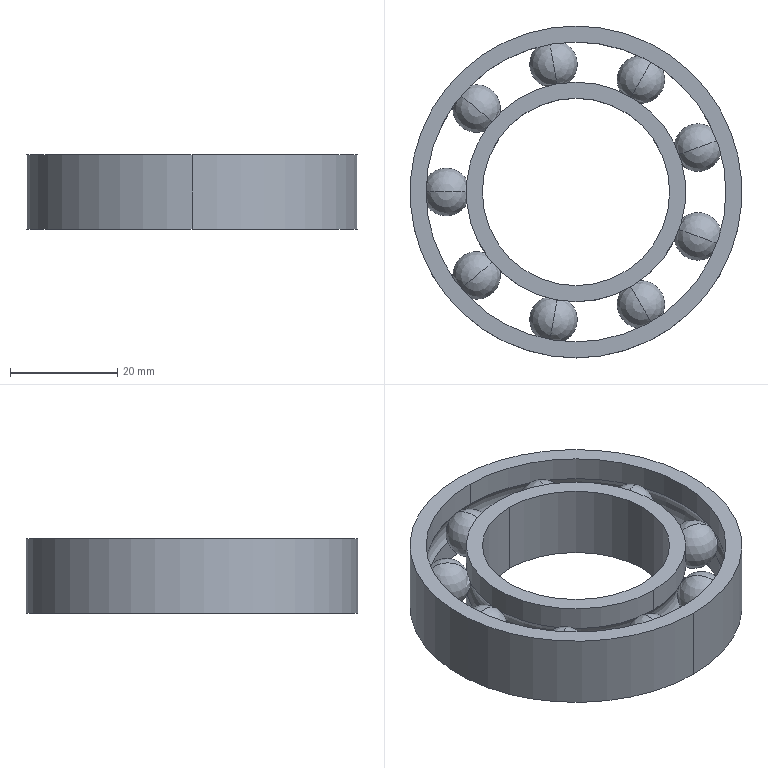Part | NX | features BREP 11 | 11 solids | 38 faces | box 62 x 62 x 14 mm | volume 15463 mm3 | sphere 18 | cylinder 12 | plane 4 | torus 4 | commonest cylinder face diameters 41 x4 56 x4 35 x2 62 x2
STEP:
#1=CARTESIAN_POINT('',(-18.577,15.588,-4.5));
#2=VERTEX_POINT('',#1);
#3=CARTESIAN_POINT('',(-18.577,15.588,4.5));
#4=VERTEX_POINT('',#3);
#5=CARTESIAN_POINT('',(-18.577,15.588,0.));
#6=DIRECTION('',(-0.6428,-0.766,0.));
#7=DIRECTION('',(0.,0.,-1.));
#8=AXIS2_PLACEMENT_3D('',#5,#6,#7);
#9=CIRCLE('',#8,4.5);
#10=EDGE_CURVE('',#2,#4,#9,.T.);
#11=ORIENTED_EDGE('',*,*,#10,.F.);
#12=CARTESIAN_POINT('',(-18.577,15.588,0.));
#13=DIRECTION('',(0.6428,0.766,0.));
#14=DIRECTION('',(0.,0.,-1.));
#15=AXIS2_PLACEMENT_3D('',#12,#13,#14);
#16=CIRCLE('',#15,4.5);
#17=EDGE_CURVE('',#2,#4,#16,.T.);
#18=ORIENTED_EDGE('',*,*,#17,.T.);
#19=EDGE_LOOP('',(#11,#18));
#20=FACE_BOUND('',#19,.T.);
#21=CARTESIAN_POINT('',(-18.577,15.588,0.));
#22=DIRECTION('',(0.,0.,-1.));
#23=DIRECTION('',(-0.766,0.6428,0.));
#24=AXIS2_PLACEMENT_3D('',#21,#22,#23);
#25=SPHERICAL_SURFACE('',#24,4.5);
#26=ADVANCED_FACE('',(#20),#25,.T.);
#27=ORIENTED_EDGE('',*,*,#10,.T.);
#28=ORIENTED_EDGE('',*,*,#17,.F.);
#29=EDGE_LOOP('',(#27,#28));
#30=FACE_BOUND('',#29,.T.);
#31=CARTESIAN_POINT('',(-18.577,15.588,0.));
#32=DIRECTION('',(0.,0.,-1.));
#33=DIRECTION('',(-0.766,0.6428,0.));
#34=AXIS2_PLACEMENT_3D('',#31,#32,#33);
#35=SPHERICAL_SURFACE('',#34,4.5);
#36=ADVANCED_FACE('',(#30),#35,.T.);
#37=CLOSED_SHELL('',(#26,#36));
#38=MANIFOLD_SOLID_BREP('',#37);
#39=CARTESIAN_POINT('',(-4.211,23.882,-4.5));
#40=VERTEX_POINT('',#39);
#41=CARTESIAN_POINT('',(-4.211,23.882,4.5));
#42=VERTEX_POINT('',#41);
#43=CARTESIAN_POINT('',(-4.211,23.882,0.));
#44=DIRECTION('',(-0.9848,-0.1736,0.));
#45=DIRECTION('',(0.,0.,-1.));
#46=AXIS2_PLACEMENT_3D('',#43,#44,#45);
#47=CIRCLE('',#46,4.5);
#48=EDGE_CURVE('',#40,#42,#47,.T.);
#49=ORIENTED_EDGE('',*,*,#48,.F.);
#50=CARTESIAN_POINT('',(-4.211,23.882,0.));
#51=DIRECTION('',(0.9848,0.1736,0.));
#52=DIRECTION('',(0.,0.,-1.));
#53=AXIS2_PLACEMENT_3D('',#50,#51,#52);
#54=CIRCLE('',#53,4.5);
#55=EDGE_CURVE('',#40,#42,#54,.T.);
#56=ORIENTED_EDGE('',*,*,#55,.T.);
#57=EDGE_LOOP('',(#49,#56));
#58=FACE_BOUND('',#57,.T.);
#59=CARTESIAN_POINT('',(-4.211,23.882,0.));
#60=DIRECTION('',(0.,0.,-1.));
#61=DIRECTION('',(-0.1736,0.9848,0.));
#62=AXIS2_PLACEMENT_3D('',#59,#60,#61);
#63=SPHERICAL_SURFACE('',#62,4.5);
#64=ADVANCED_FACE('',(#58),#63,.T.);
#65=ORIENTED_EDGE('',*,*,#48,.T.);
#66=ORIENTED_EDGE('',*,*,#55,.F.);
#67=EDGE_LOOP('',(#65,#66));
#68=FACE_BOUND('',#67,.T.);
#69=CARTESIAN_POINT('',(-4.211,23.882,0.));
#70=DIRECTION('',(0.,0.,-1.));
#71=DIRECTION('',(-0.1736,0.9848,0.));
#72=AXIS2_PLACEMENT_3D('',#69,#70,#71);
#73=SPHERICAL_SURFACE('',#72,4.5);
#74=ADVANCED_FACE('',(#68),#73,.T.);
#75=CLOSED_SHELL('',(#64,#74));
#76=MANIFOLD_SOLID_BREP('',#75);
#77=CARTESIAN_POINT('',(0.,31.,-7.));
#78=VERTEX_POINT('',#77);
#79=CARTESIAN_POINT('',(0.,-31.,-7.));
#80=VERTEX_POINT('',#79);
#81=CARTESIAN_POINT('',(0.,0.,-7.));
#82=DIRECTION('',(0.,0.,1.));
#83=DIRECTION('',(0.,1.,0.));
#84=AXIS2_PLACEMENT_3D('',#81,#82,#83);
#85=CIRCLE('',#84,31.);
#86=EDGE_CURVE('',#78,#80,#85,.T.);
#87=ORIENTED_EDGE('',*,*,#86,.T.);
#88=CARTESIAN_POINT('',(0.,-31.,7.));
#89=VERTEX_POINT('',#88);
#90=CARTESIAN_POINT('',(0.,-31.,-7.));
#91=DIRECTION('',(0.,0.,1.));
#92=VECTOR('',#91,1000.);
#93=LINE('',#90,#92);
#94=EDGE_CURVE('',#80,#89,#93,.T.);
#95=ORIENTED_EDGE('',*,*,#94,.T.);
#96=CARTESIAN_POINT('',(0.,31.,7.));
#97=VERTEX_POINT('',#96);
#98=CARTESIAN_POINT('',(0.,0.,7.));
#99=DIRECTION('',(0.,0.,1.));
#100=DIRECTION('',(0.,1.,0.));
#101=AXIS2_PLACEMENT_3D('',#98,#99,#100);
#102=CIRCLE('',#101,31.);
#103=EDGE_CURVE('',#97,#89,#102,.T.);
#104=ORIENTED_EDGE('',*,*,#103,.F.);
#105=CARTESIAN_POINT('',(0.,31.,-7.));
#106=DIRECTION('',(0.,0.,1.));
#107=VECTOR('',#106,1000.);
#108=LINE('',#105,#107);
#109=EDGE_CURVE('',#78,#97,#108,.T.);
#110=ORIENTED_EDGE('',*,*,#109,.F.);
#111=EDGE_LOOP('',(#87,#95,#104,#110));
#112=FACE_BOUND('',#111,.T.);
#113=CARTESIAN_POINT('',(0.,0.,7.7));
#114=DIRECTION('',(0.,0.,-1.));
#115=DIRECTION('',(0.,1.,0.));
#116=AXIS2_PLACEMENT_3D('',#113,#114,#115);
#117=CYLINDRICAL_SURFACE('',#116,31.);
#118=ADVANCED_FACE('',(#112),#117,.T.);
#119=CARTESIAN_POINT('',(0.,0.,7.));
#120=DIRECTION('',(0.,0.,-1.));
#121=DIRECTION('',(0.,1.,0.));
#122=AXIS2_PLACEMENT_3D('',#119,#120,#121);
#123=CIRCLE('',#122,31.);
#124=EDGE_CURVE('',#97,#89,#123,.T.);
#125=ORIENTED_EDGE('',*,*,#124,.T.);
#126=ORIENTED_EDGE('',*,*,#94,.F.);
#127=CARTESIAN_POINT('',(0.,0.,-7.));
#128=DIRECTION('',(0.,0.,-1.));
#129=DIRECTION('',(0.,1.,0.));
#130=AXIS2_PLACEMENT_3D('',#127,#128,#129);
#131=CIRCLE('',#130,31.);
#132=EDGE_CURVE('',#78,#80,#131,.T.);
#133=ORIENTED_EDGE('',*,*,#132,.F.);
#134=ORIENTED_EDGE('',*,*,#109,.T.);
#135=EDGE_LOOP('',(#125,#126,#133,#134));
#136=FACE_BOUND('',#135,.T.);
#137=CARTESIAN_POINT('',(0.,0.,7.7));
#138=DIRECTION('',(0.,0.,-1.));
#139=DIRECTION('',(0.,1.,0.));
#140=AXIS2_PLACEMENT_3D('',#137,#138,#139);
#141=CYLINDRICAL_SURFACE('',#140,31.);
#142=ADVANCED_FACE('',(#136),#141,.T.);
#143=ORIENTED_EDGE('',*,*,#86,.F.);
#144=ORIENTED_EDGE('',*,*,#132,.T.);
#145=EDGE_LOOP('',(#143,#144));
#146=FACE_BOUND('',#145,.T.);
#147=CARTESIAN_POINT('',(0.,28.,-7.));
#148=VERTEX_POINT('',#147);
#149=CARTESIAN_POINT('',(0.,-28.,-7.));
#150=VERTEX_POINT('',#149);
#151=CARTESIAN_POINT('',(0.,0.,-7.));
#152=DIRECTION('',(0.,0.,-1.));
#153=DIRECTION('',(0.,1.,0.));
#154=AXIS2_PLACEMENT_3D('',#151,#152,#153);
#155=CIRCLE('',#154,28.);
#156=EDGE_CURVE('',#148,#150,#155,.T.);
#157=ORIENTED_EDGE('',*,*,#156,.F.);
#158=CARTESIAN_POINT('',(0.,0.,-7.));
#159=DIRECTION('',(0.,0.,1.));
#160=DIRECTION('',(0.,1.,0.));
#161=AXIS2_PLACEMENT_3D('',#158,#159,#160);
#162=CIRCLE('',#161,28.);
#163=EDGE_CURVE('',#148,#150,#162,.T.);
#164=ORIENTED_EDGE('',*,*,#163,.T.);
#165=EDGE_LOOP('',(#157,#164));
#166=FACE_BOUND('',#165,.T.);
#167=CARTESIAN_POINT('',(0.,0.,-7.));
#168=DIRECTION('',(0.,0.,-1.));
#169=DIRECTION('',(0.,1.,0.));
#170=AXIS2_PLACEMENT_3D('',#167,#168,#169);
#171=PLANE('',#170);
#172=ADVANCED_FACE('',(#146,#166),#171,.T.);
#173=CARTESIAN_POINT('',(0.,28.,-2.487));
#174=VERTEX_POINT('',#173);
#175=CARTESIAN_POINT('',(0.,-28.,-2.487));
#176=VERTEX_POINT('',#175);
#177=CARTESIAN_POINT('',(0.,0.,-2.487));
#178=DIRECTION('',(0.,0.,1.));
#179=DIRECTION('',(0.,1.,0.));
#180=AXIS2_PLACEMENT_3D('',#177,#178,#179);
#181=CIRCLE('',#180,28.);
#182=EDGE_CURVE('',#174,#176,#181,.T.);
#183=ORIENTED_EDGE('',*,*,#182,.T.);
#184=CARTESIAN_POINT('',(0.,-28.,-2.487));
#185=DIRECTION('',(0.,0.,-1.));
#186=VECTOR('',#185,1000.);
#187=LINE('',#184,#186);
#188=EDGE_CURVE('',#176,#150,#187,.T.);
#189=ORIENTED_EDGE('',*,*,#188,.T.);
#190=ORIENTED_EDGE('',*,*,#163,.F.);
#191=CARTESIAN_POINT('',(0.,28.,-2.487));
#192=DIRECTION('',(0.,0.,-1.));
#193=VECTOR('',#192,1000.);
#194=LINE('',#191,#193);
#195=EDGE_CURVE('',#174,#148,#194,.T.);
#196=ORIENTED_EDGE('',*,*,#195,.F.);
#197=EDGE_LOOP('',(#183,#189,#190,#196));
#198=FACE_BOUND('',#197,.T.);
#199=CARTESIAN_POINT('',(0.,0.,7.7));
#200=DIRECTION('',(0.,0.,-1.));
#201=DIRECTION('',(0.,1.,0.));
#202=AXIS2_PLACEMENT_3D('',#199,#200,#201);
#203=CYLINDRICAL_SURFACE('',#202,28.);
#204=ADVANCED_FACE('',(#198),#203,.F.);
#205=ORIENTED_EDGE('',*,*,#156,.T.);
#206=ORIENTED_EDGE('',*,*,#188,.F.);
#207=CARTESIAN_POINT('',(0.,0.,-2.487));
#208=DIRECTION('',(0.,0.,-1.));
#209=DIRECTION('',(0.,1.,0.));
#210=AXIS2_PLACEMENT_3D('',#207,#208,#209);
#211=CIRCLE('',#210,28.);
#212=EDGE_CURVE('',#174,#176,#211,.T.);
#213=ORIENTED_EDGE('',*,*,#212,.F.);
#214=ORIENTED_EDGE('',*,*,#195,.T.);
#215=EDGE_LOOP('',(#205,#206,#213,#214));
#216=FACE_BOUND('',#215,.T.);
#217=CARTESIAN_POINT('',(0.,0.,7.7));
#218=DIRECTION('',(0.,0.,-1.));
#219=DIRECTION('',(0.,1.,0.));
#220=AXIS2_PLACEMENT_3D('',#217,#218,#219);
#221=CYLINDRICAL_SURFACE('',#220,28.);
#222=ADVANCED_FACE('',(#216),#221,.F.);
#223=ORIENTED_EDGE('',*,*,#212,.T.);
#224=CARTESIAN_POINT('',(0.,-28.,2.487));
#225=VERTEX_POINT('',#224);
#226=CARTESIAN_POINT('',(0.,-24.25,0.));
#227=DIRECTION('',(1.,0.,0.));
#228=DIRECTION('',(0.,-0.8333,0.5528));
#229=AXIS2_PLACEMENT_3D('',#226,#227,#228);
#230=CIRCLE('',#229,4.5);
#231=EDGE_CURVE('',#176,#225,#230,.F.);
#232=ORIENTED_EDGE('',*,*,#231,.T.);
#233=CARTESIAN_POINT('',(0.,28.,2.487));
#234=VERTEX_POINT('',#233);
#235=CARTESIAN_POINT('',(0.,0.,2.487));
#236=DIRECTION('',(0.,0.,-1.));
#237=DIRECTION('',(0.,1.,0.));
#238=AXIS2_PLACEMENT_3D('',#235,#236,#237);
#239=CIRCLE('',#238,28.);
#240=EDGE_CURVE('',#234,#225,#239,.T.);
#241=ORIENTED_EDGE('',*,*,#240,.F.);
#242=CARTESIAN_POINT('',(0.,24.25,0.));
#243=DIRECTION('',(-1.,0.,0.));
#244=DIRECTION('',(0.,0.8333,0.5528));
#245=AXIS2_PLACEMENT_3D('',#242,#243,#244);
#246=CIRCLE('',#245,4.5);
#247=EDGE_CURVE('',#174,#234,#246,.F.);
#248=ORIENTED_EDGE('',*,*,#247,.F.);
#249=EDGE_LOOP('',(#223,#232,#241,#248));
#250=FACE_BOUND('',#249,.T.);
#251=CARTESIAN_POINT('',(0.,0.,0.));
#252=DIRECTION('',(0.,0.,-1.));
#253=DIRECTION('',(0.,1.,0.));
#254=AXIS2_PLACEMENT_3D('',#251,#252,#253);
#255=TOROIDAL_SURFACE('',#254,24.25,4.5);
#256=ADVANCED_FACE('',(#250),#255,.F.);
#257=CARTESIAN_POINT('',(0.,0.,2.487));
#258=DIRECTION('',(0.,0.,1.));
#259=DIRECTION('',(0.,1.,0.));
#260=AXIS2_PLACEMENT_3D('',#257,#258,#259);
#261=CIRCLE('',#260,28.);
#262=EDGE_CURVE('',#234,#225,#261,.T.);
#263=ORIENTED_EDGE('',*,*,#262,.T.);
#264=ORIENTED_EDGE('',*,*,#231,.F.);
#265=ORIENTED_EDGE('',*,*,#182,.F.);
#266=ORIENTED_EDGE('',*,*,#247,.T.);
#267=EDGE_LOOP('',(#263,#264,#265,#266));
#268=FACE_BOUND('',#267,.T.);
#269=CARTESIAN_POINT('',(0.,0.,0.));
#270=DIRECTION('',(0.,0.,-1.));
#271=DIRECTION('',(0.,1.,0.));
#272=AXIS2_PLACEMENT_3D('',#269,#270,#271);
#273=TOROIDAL_SURFACE('',#272,24.25,4.5);
#274=ADVANCED_FACE('',(#268),#273,.F.);
#275=CARTESIAN_POINT('',(0.,28.,7.));
#276=VERTEX_POINT('',#275);
#277=CARTESIAN_POINT('',(0.,-28.,7.));
#278=VERTEX_POINT('',#277);
#279=CARTESIAN_POINT('',(0.,0.,7.));
#280=DIRECTION('',(0.,0.,1.));
#281=DIRECTION('',(0.,1.,0.));
#282=AXIS2_PLACEMENT_3D('',#279,#280,#281);
#283=CIRCLE('',#282,28.);
#284=EDGE_CURVE('',#276,#278,#283,.T.);
#285=ORIENTED_EDGE('',*,*,#284,.T.);
#286=CARTESIAN_POINT('',(0.,-28.,7.));
#287=DIRECTION('',(0.,0.,-1.));
#288=VECTOR('',#287,1000.);
#289=LINE('',#286,#288);
#290=EDGE_CURVE('',#278,#225,#289,.T.);
#291=ORIENTED_EDGE('',*,*,#290,.T.);
#292=ORIENTED_EDGE('',*,*,#262,.F.);
#293=CARTESIAN_POINT('',(0.,28.,7.));
#294=DIRECTION('',(0.,0.,-1.));
#295=VECTOR('',#294,1000.);
#296=LINE('',#293,#295);
#297=EDGE_CURVE('',#276,#234,#296,.T.);
#298=ORIENTED_EDGE('',*,*,#297,.F.);
#299=EDGE_LOOP('',(#285,#291,#292,#298));
#300=FACE_BOUND('',#299,.T.);
#301=CARTESIAN_POINT('',(0.,0.,7.7));
#302=DIRECTION('',(0.,0.,-1.));
#303=DIRECTION('',(0.,1.,0.));
#304=AXIS2_PLACEMENT_3D('',#301,#302,#303);
#305=CYLINDRICAL_SURFACE('',#304,28.);
#306=ADVANCED_FACE('',(#300),#305,.F.);
#307=ORIENTED_EDGE('',*,*,#240,.T.);
#308=ORIENTED_EDGE('',*,*,#290,.F.);
#309=CARTESIAN_POINT('',(0.,0.,7.));
#310=DIRECTION('',(0.,0.,-1.));
#311=DIRECTION('',(0.,1.,0.));
#312=AXIS2_PLACEMENT_3D('',#309,#310,#311);
#313=CIRCLE('',#312,28.);
#314=EDGE_CURVE('',#276,#278,#313,.T.);
#315=ORIENTED_EDGE('',*,*,#314,.F.);
#316=ORIENTED_EDGE('',*,*,#297,.T.);
#317=EDGE_LOOP('',(#307,#308,#315,#316));
#318=FACE_BOUND('',#317,.T.);
#319=CARTESIAN_POINT('',(0.,0.,7.7));
#320=DIRECTION('',(0.,0.,-1.));
#321=DIRECTION('',(0.,1.,0.));
#322=AXIS2_PLACEMENT_3D('',#319,#320,#321);
#323=CYLINDRICAL_SURFACE('',#322,28.);
#324=ADVANCED_FACE('',(#318),#323,.F.);
#325=ORIENTED_EDGE('',*,*,#124,.F.);
#326=ORIENTED_EDGE('',*,*,#103,.T.);
#327=EDGE_LOOP('',(#325,#326));
#328=FACE_BOUND('',#327,.T.);
#329=ORIENTED_EDGE('',*,*,#284,.F.);
#330=ORIENTED_EDGE('',*,*,#314,.T.);
#331=EDGE_LOOP('',(#329,#330));
#332=FACE_BOUND('',#331,.T.);
#333=CARTESIAN_POINT('',(0.,0.,7.));
#334=DIRECTION('',(0.,0.,-1.));
#335=DIRECTION('',(0.,1.,0.));
#336=AXIS2_PLACEMENT_3D('',#333,#334,#335);
#337=PLANE('',#336);
#338=ADVANCED_FACE('',(#328,#332),#337,.F.);
#339=CLOSED_SHELL('',(#118,#142,#172,#204,#222,#256,#274,#306,#324,#338));
#340=MANIFOLD_SOLID_BREP('',#339);
#341=CARTESIAN_POINT('',(12.125,21.001,4.5));
#342=VERTEX_POINT('',#341);
#343=CARTESIAN_POINT('',(12.125,21.001,-4.5));
#344=VERTEX_POINT('',#343);
#345=CARTESIAN_POINT('',(12.125,21.001,0.));
#346=DIRECTION('',(-0.866,0.5,0.));
#347=DIRECTION('',(0.,0.,-1.));
#348=AXIS2_PLACEMENT_3D('',#345,#346,#347);
#349=CIRCLE('',#348,4.5);
#350=EDGE_CURVE('',#342,#344,#349,.F.);
#351=ORIENTED_EDGE('',*,*,#350,.T.);
#352=CARTESIAN_POINT('',(12.125,21.001,0.));
#353=DIRECTION('',(0.866,-0.5,0.));
#354=DIRECTION('',(0.,0.,-1.));
#355=AXIS2_PLACEMENT_3D('',#352,#353,#354);
#356=CIRCLE('',#355,4.5);
#357=EDGE_CURVE('',#342,#344,#356,.F.);
#358=ORIENTED_EDGE('',*,*,#357,.F.);
#359=EDGE_LOOP('',(#351,#358));
#360=FACE_BOUND('',#359,.T.);
#361=CARTESIAN_POINT('',(12.125,21.001,0.));
#362=DIRECTION('',(0.,0.,-1.));
#363=DIRECTION('',(0.5,0.866,0.));
#364=AXIS2_PLACEMENT_3D('',#361,#362,#363);
#365=SPHERICAL_SURFACE('',#364,4.5);
#366=ADVANCED_FACE('',(#360),#365,.T.);
#367=ORIENTED_EDGE('',*,*,#350,.F.);
#368=ORIENTED_EDGE('',*,*,#357,.T.);
#369=EDGE_LOOP('',(#367,#368));
#370=FACE_BOUND('',#369,.T.);
#371=CARTESIAN_POINT('',(12.125,21.001,0.));
#372=DIRECTION('',(0.,0.,-1.));
#373=DIRECTION('',(0.5,0.866,0.));
#374=AXIS2_PLACEMENT_3D('',#371,#372,#373);
#375=SPHERICAL_SURFACE('',#374,4.5);
#376=ADVANCED_FACE('',(#370),#375,.T.);
#377=CLOSED_SHELL('',(#366,#376));
#378=MANIFOLD_SOLID_BREP('',#377);
#379=CARTESIAN_POINT('',(0.,20.5,2.487));
#380=VERTEX_POINT('',#379);
#381=CARTESIAN_POINT('',(0.,-20.5,2.487));
#382=VERTEX_POINT('',#381);
#383=CARTESIAN_POINT('',(0.,0.,2.487));
#384=DIRECTION('',(0.,0.,1.));
#385=DIRECTION('',(0.,1.,0.));
#386=AXIS2_PLACEMENT_3D('',#383,#384,#385);
#387=CIRCLE('',#386,20.5);
#388=EDGE_CURVE('',#380,#382,#387,.T.);
#389=ORIENTED_EDGE('',*,*,#388,.T.);
#390=CARTESIAN_POINT('',(0.,-20.5,7.));
#391=VERTEX_POINT('',#390);
#392=CARTESIAN_POINT('',(0.,-20.5,2.487));
#393=DIRECTION('',(0.,0.,1.));
#394=VECTOR('',#393,1000.);
#395=LINE('',#392,#394);
#396=EDGE_CURVE('',#382,#391,#395,.T.);
#397=ORIENTED_EDGE('',*,*,#396,.T.);
#398=CARTESIAN_POINT('',(0.,20.5,7.));
#399=VERTEX_POINT('',#398);
#400=CARTESIAN_POINT('',(0.,0.,7.));
#401=DIRECTION('',(0.,0.,1.));
#402=DIRECTION('',(0.,1.,0.));
#403=AXIS2_PLACEMENT_3D('',#400,#401,#402);
#404=CIRCLE('',#403,20.5);
#405=EDGE_CURVE('',#399,#391,#404,.T.);
#406=ORIENTED_EDGE('',*,*,#405,.F.);
#407=CARTESIAN_POINT('',(0.,20.5,2.487));
#408=DIRECTION('',(0.,0.,1.));
#409=VECTOR('',#408,1000.);
#410=LINE('',#407,#409);
#411=EDGE_CURVE('',#380,#399,#410,.T.);
#412=ORIENTED_EDGE('',*,*,#411,.F.);
#413=EDGE_LOOP('',(#389,#397,#406,#412));
#414=FACE_BOUND('',#413,.T.);
#415=CARTESIAN_POINT('',(0.,0.,7.7));
#416=DIRECTION('',(0.,0.,-1.));
#417=DIRECTION('',(0.,1.,0.));
#418=AXIS2_PLACEMENT_3D('',#415,#416,#417);
#419=CYLINDRICAL_SURFACE('',#418,20.5);
#420=ADVANCED_FACE('',(#414),#419,.T.);
#421=CARTESIAN_POINT('',(0.,0.,7.));
#422=DIRECTION('',(0.,0.,-1.));
#423=DIRECTION('',(0.,1.,0.));
#424=AXIS2_PLACEMENT_3D('',#421,#422,#423);
#425=CIRCLE('',#424,20.5);
#426=EDGE_CURVE('',#399,#391,#425,.T.);
#427=ORIENTED_EDGE('',*,*,#426,.T.);
#428=ORIENTED_EDGE('',*,*,#396,.F.);
#429=CARTESIAN_POINT('',(0.,0.,2.487));
#430=DIRECTION('',(0.,0.,-1.));
#431=DIRECTION('',(0.,1.,0.));
#432=AXIS2_PLACEMENT_3D('',#429,#430,#431);
#433=CIRCLE('',#432,20.5);
#434=EDGE_CURVE('',#380,#382,#433,.T.);
#435=ORIENTED_EDGE('',*,*,#434,.F.);
#436=ORIENTED_EDGE('',*,*,#411,.T.);
#437=EDGE_LOOP('',(#427,#428,#435,#436));
#438=FACE_BOUND('',#437,.T.);
#439=CARTESIAN_POINT('',(0.,0.,7.7));
#440=DIRECTION('',(0.,0.,-1.));
#441=DIRECTION('',(0.,1.,0.));
#442=AXIS2_PLACEMENT_3D('',#439,#440,#441);
#443=CYLINDRICAL_SURFACE('',#442,20.5);
#444=ADVANCED_FACE('',(#438),#443,.T.);
#445=ORIENTED_EDGE('',*,*,#434,.T.);
#446=CARTESIAN_POINT('',(0.,-20.5,-2.487));
#447=VERTEX_POINT('',#446);
#448=CARTESIAN_POINT('',(0.,-24.25,0.));
#449=DIRECTION('',(1.,0.,0.));
#450=DIRECTION('',(0.,0.8333,-0.5528));
#451=AXIS2_PLACEMENT_3D('',#448,#449,#450);
#452=CIRCLE('',#451,4.5);
#453=EDGE_CURVE('',#382,#447,#452,.F.);
#454=ORIENTED_EDGE('',*,*,#453,.T.);
#455=CARTESIAN_POINT('',(0.,20.5,-2.487));
#456=VERTEX_POINT('',#455);
#457=CARTESIAN_POINT('',(0.,0.,-2.487));
#458=DIRECTION('',(0.,0.,-1.));
#459=DIRECTION('',(0.,1.,0.));
#460=AXIS2_PLACEMENT_3D('',#457,#458,#459);
#461=CIRCLE('',#460,20.5);
#462=EDGE_CURVE('',#456,#447,#461,.T.);
#463=ORIENTED_EDGE('',*,*,#462,.F.);
#464=CARTESIAN_POINT('',(0.,24.25,0.));
#465=DIRECTION('',(-1.,0.,0.));
#466=DIRECTION('',(0.,-0.8333,-0.5528));
#467=AXIS2_PLACEMENT_3D('',#464,#465,#466);
#468=CIRCLE('',#467,4.5);
#469=EDGE_CURVE('',#380,#456,#468,.F.);
#470=ORIENTED_EDGE('',*,*,#469,.F.);
#471=EDGE_LOOP('',(#445,#454,#463,#470));
#472=FACE_BOUND('',#471,.T.);
#473=CARTESIAN_POINT('',(0.,0.,0.));
#474=DIRECTION('',(0.,0.,-1.));
#475=DIRECTION('',(0.,1.,0.));
#476=AXIS2_PLACEMENT_3D('',#473,#474,#475);
#477=TOROIDAL_SURFACE('',#476,24.25,4.5);
#478=ADVANCED_FACE('',(#472),#477,.F.);
#479=CARTESIAN_POINT('',(0.,0.,-2.487));
#480=DIRECTION('',(0.,0.,1.));
#481=DIRECTION('',(0.,1.,0.));
#482=AXIS2_PLACEMENT_3D('',#479,#480,#481);
#483=CIRCLE('',#482,20.5);
#484=EDGE_CURVE('',#456,#447,#483,.T.);
#485=ORIENTED_EDGE('',*,*,#484,.T.);
#486=ORIENTED_EDGE('',*,*,#453,.F.);
#487=ORIENTED_EDGE('',*,*,#388,.F.);
#488=ORIENTED_EDGE('',*,*,#469,.T.);
#489=EDGE_LOOP('',(#485,#486,#487,#488));
#490=FACE_BOUND('',#489,.T.);
#491=CARTESIAN_POINT('',(0.,0.,0.));
#492=DIRECTION('',(0.,0.,-1.));
#493=DIRECTION('',(0.,1.,0.));
#494=AXIS2_PLACEMENT_3D('',#491,#492,#493);
#495=TOROIDAL_SURFACE('',#494,24.25,4.5);
#496=ADVANCED_FACE('',(#490),#495,.F.);
#497=CARTESIAN_POINT('',(0.,20.5,-7.));
#498=VERTEX_POINT('',#497);
#499=CARTESIAN_POINT('',(0.,-20.5,-7.));
#500=VERTEX_POINT('',#499);
#501=CARTESIAN_POINT('',(0.,0.,-7.));
#502=DIRECTION('',(0.,0.,1.));
#503=DIRECTION('',(0.,1.,0.));
#504=AXIS2_PLACEMENT_3D('',#501,#502,#503);
#505=CIRCLE('',#504,20.5);
#506=EDGE_CURVE('',#498,#500,#505,.T.);
#507=ORIENTED_EDGE('',*,*,#506,.T.);
#508=CARTESIAN_POINT('',(0.,-20.5,-7.));
#509=DIRECTION('',(0.,0.,1.));
#510=VECTOR('',#509,1000.);
#511=LINE('',#508,#510);
#512=EDGE_CURVE('',#500,#447,#511,.T.);
#513=ORIENTED_EDGE('',*,*,#512,.T.);
#514=ORIENTED_EDGE('',*,*,#484,.F.);
#515=CARTESIAN_POINT('',(0.,20.5,-7.));
#516=DIRECTION('',(0.,0.,1.));
#517=VECTOR('',#516,1000.);
#518=LINE('',#515,#517);
#519=EDGE_CURVE('',#498,#456,#518,.T.);
#520=ORIENTED_EDGE('',*,*,#519,.F.);
#521=EDGE_LOOP('',(#507,#513,#514,#520));
#522=FACE_BOUND('',#521,.T.);
#523=CARTESIAN_POINT('',(0.,0.,7.7));
#524=DIRECTION('',(0.,0.,-1.));
#525=DIRECTION('',(0.,1.,0.));
#526=AXIS2_PLACEMENT_3D('',#523,#524,#525);
#527=CYLINDRICAL_SURFACE('',#526,20.5);
#528=ADVANCED_FACE('',(#522),#527,.T.);
#529=ORIENTED_EDGE('',*,*,#462,.T.);
#530=ORIENTED_EDGE('',*,*,#512,.F.);
#531=CARTESIAN_POINT('',(0.,0.,-7.));
#532=DIRECTION('',(0.,0.,-1.));
#533=DIRECTION('',(0.,1.,0.));
#534=AXIS2_PLACEMENT_3D('',#531,#532,#533);
#535=CIRCLE('',#534,20.5);
#536=EDGE_CURVE('',#498,#500,#535,.T.);
#537=ORIENTED_EDGE('',*,*,#536,.F.);
#538=ORIENTED_EDGE('',*,*,#519,.T.);
#539=EDGE_LOOP('',(#529,#530,#537,#538));
#540=FACE_BOUND('',#539,.T.);
#541=CARTESIAN_POINT('',(0.,0.,7.7));
#542=DIRECTION('',(0.,0.,-1.));
#543=DIRECTION('',(0.,1.,0.));
#544=AXIS2_PLACEMENT_3D('',#541,#542,#543);
#545=CYLINDRICAL_SURFACE('',#544,20.5);
#546=ADVANCED_FACE('',(#540),#545,.T.);
#547=ORIENTED_EDGE('',*,*,#506,.F.);
#548=ORIENTED_EDGE('',*,*,#536,.T.);
#549=EDGE_LOOP('',(#547,#548));
#550=FACE_BOUND('',#549,.T.);
#551=CARTESIAN_POINT('',(0.,17.5,-7.));
#552=VERTEX_POINT('',#551);
#553=CARTESIAN_POINT('',(0.,-17.5,-7.));
#554=VERTEX_POINT('',#553);
#555=CARTESIAN_POINT('',(0.,0.,-7.));
#556=DIRECTION('',(0.,0.,-1.));
#557=DIRECTION('',(0.,1.,0.));
#558=AXIS2_PLACEMENT_3D('',#555,#556,#557);
#559=CIRCLE('',#558,17.5);
#560=EDGE_CURVE('',#552,#554,#559,.T.);
#561=ORIENTED_EDGE('',*,*,#560,.F.);
#562=CARTESIAN_POINT('',(0.,0.,-7.));
#563=DIRECTION('',(0.,0.,1.));
#564=DIRECTION('',(0.,1.,0.));
#565=AXIS2_PLACEMENT_3D('',#562,#563,#564);
#566=CIRCLE('',#565,17.5);
#567=EDGE_CURVE('',#552,#554,#566,.T.);
#568=ORIENTED_EDGE('',*,*,#567,.T.);
#569=EDGE_LOOP('',(#561,#568));
#570=FACE_BOUND('',#569,.T.);
#571=CARTESIAN_POINT('',(0.,0.,-7.));
#572=DIRECTION('',(0.,0.,-1.));
#573=DIRECTION('',(0.,1.,0.));
#574=AXIS2_PLACEMENT_3D('',#571,#572,#573);
#575=PLANE('',#574);
#576=ADVANCED_FACE('',(#550,#570),#575,.T.);
#577=CARTESIAN_POINT('',(0.,17.5,7.));
#578=VERTEX_POINT('',#577);
#579=CARTESIAN_POINT('',(0.,-17.5,7.));
#580=VERTEX_POINT('',#579);
#581=CARTESIAN_POINT('',(0.,0.,7.));
#582=DIRECTION('',(0.,0.,1.));
#583=DIRECTION('',(0.,1.,0.));
#584=AXIS2_PLACEMENT_3D('',#581,#582,#583);
#585=CIRCLE('',#584,17.5);
#586=EDGE_CURVE('',#578,#580,#585,.T.);
#587=ORIENTED_EDGE('',*,*,#586,.T.);
#588=CARTESIAN_POINT('',(0.,-17.5,7.));
#589=DIRECTION('',(0.,0.,-1.));
#590=VECTOR('',#589,1000.);
#591=LINE('',#588,#590);
#592=EDGE_CURVE('',#580,#554,#591,.T.);
#593=ORIENTED_EDGE('',*,*,#592,.T.);
#594=ORIENTED_EDGE('',*,*,#567,.F.);
#595=CARTESIAN_POINT('',(0.,17.5,7.));
#596=DIRECTION('',(0.,0.,-1.));
#597=VECTOR('',#596,1000.);
#598=LINE('',#595,#597);
#599=EDGE_CURVE('',#578,#552,#598,.T.);
#600=ORIENTED_EDGE('',*,*,#599,.F.);
#601=EDGE_LOOP('',(#587,#593,#594,#600));
#602=FACE_BOUND('',#601,.T.);
#603=CARTESIAN_POINT('',(0.,0.,7.7));
#604=DIRECTION('',(0.,0.,-1.));
#605=DIRECTION('',(0.,1.,0.));
#606=AXIS2_PLACEMENT_3D('',#603,#604,#605);
#607=CYLINDRICAL_SURFACE('',#606,17.5);
#608=ADVANCED_FACE('',(#602),#607,.F.);
#609=ORIENTED_EDGE('',*,*,#560,.T.);
#610=ORIENTED_EDGE('',*,*,#592,.F.);
#611=CARTESIAN_POINT('',(0.,0.,7.));
#612=DIRECTION('',(0.,0.,-1.));
#613=DIRECTION('',(0.,1.,0.));
#614=AXIS2_PLACEMENT_3D('',#611,#612,#613);
#615=CIRCLE('',#614,17.5);
#616=EDGE_CURVE('',#578,#580,#615,.T.);
#617=ORIENTED_EDGE('',*,*,#616,.F.);
#618=ORIENTED_EDGE('',*,*,#599,.T.);
#619=EDGE_LOOP('',(#609,#610,#617,#618));
#620=FACE_BOUND('',#619,.T.);
#621=CARTESIAN_POINT('',(0.,0.,7.7));
#622=DIRECTION('',(0.,0.,-1.));
#623=DIRECTION('',(0.,1.,0.));
#624=AXIS2_PLACEMENT_3D('',#621,#622,#623);
#625=CYLINDRICAL_SURFACE('',#624,17.5);
#626=ADVANCED_FACE('',(#620),#625,.F.);
#627=ORIENTED_EDGE('',*,*,#426,.F.);
#628=ORIENTED_EDGE('',*,*,#405,.T.);
#629=EDGE_LOOP('',(#627,#628));
#630=FACE_BOUND('',#629,.T.);
#631=ORIENTED_EDGE('',*,*,#586,.F.);
#632=ORIENTED_EDGE('',*,*,#616,.T.);
#633=EDGE_LOOP('',(#631,#632));
#634=FACE_BOUND('',#633,.T.);
#635=CARTESIAN_POINT('',(0.,0.,7.));
#636=DIRECTION('',(0.,0.,-1.));
#637=DIRECTION('',(0.,1.,0.));
#638=AXIS2_PLACEMENT_3D('',#635,#636,#637);
#639=PLANE('',#638);
#640=ADVANCED_FACE('',(#630,#634),#639,.F.);
#641=CLOSED_SHELL('',(#420,#444,#478,#496,#528,#546,#576,#608,#626,#640));
#642=MANIFOLD_SOLID_BREP('',#641);
#643=CARTESIAN_POINT('',(-4.211,-23.882,-4.5));
#644=VERTEX_POINT('',#643);
#645=CARTESIAN_POINT('',(-4.211,-23.882,4.5));
#646=VERTEX_POINT('',#645);
#647=CARTESIAN_POINT('',(-4.211,-23.882,0.));
#648=DIRECTION('',(0.9848,-0.1736,0.));
#649=DIRECTION('',(0.,0.,-1.));
#650=AXIS2_PLACEMENT_3D('',#647,#648,#649);
#651=CIRCLE('',#650,4.5);
#652=EDGE_CURVE('',#644,#646,#651,.T.);
#653=ORIENTED_EDGE('',*,*,#652,.F.);
#654=CARTESIAN_POINT('',(-4.211,-23.882,0.));
#655=DIRECTION('',(-0.9848,0.1736,0.));
#656=DIRECTION('',(0.,0.,-1.));
#657=AXIS2_PLACEMENT_3D('',#654,#655,#656);
#658=CIRCLE('',#657,4.5);
#659=EDGE_CURVE('',#644,#646,#658,.T.);
#660=ORIENTED_EDGE('',*,*,#659,.T.);
#661=EDGE_LOOP('',(#653,#660));
#662=FACE_BOUND('',#661,.T.);
#663=CARTESIAN_POINT('',(-4.211,-23.882,0.));
#664=DIRECTION('',(0.,0.,-1.));
#665=DIRECTION('',(-0.1736,-0.9848,0.));
#666=AXIS2_PLACEMENT_3D('',#663,#664,#665);
#667=SPHERICAL_SURFACE('',#666,4.5);
#668=ADVANCED_FACE('',(#662),#667,.T.);
#669=ORIENTED_EDGE('',*,*,#652,.T.);
#670=ORIENTED_EDGE('',*,*,#659,.F.);
#671=EDGE_LOOP('',(#669,#670));
#672=FACE_BOUND('',#671,.T.);
#673=CARTESIAN_POINT('',(-4.211,-23.882,0.));
#674=DIRECTION('',(0.,0.,-1.));
#675=DIRECTION('',(-0.1736,-0.9848,0.));
#676=AXIS2_PLACEMENT_3D('',#673,#674,#675);
#677=SPHERICAL_SURFACE('',#676,4.5);
#678=ADVANCED_FACE('',(#672),#677,.T.);
#679=CLOSED_SHELL('',(#668,#678));
#680=MANIFOLD_SOLID_BREP('',#679);
#681=CARTESIAN_POINT('',(-18.577,-15.588,-4.5));
#682=VERTEX_POINT('',#681);
#683=CARTESIAN_POINT('',(-18.577,-15.588,4.5));
#684=VERTEX_POINT('',#683);
#685=CARTESIAN_POINT('',(-18.577,-15.588,0.));
#686=DIRECTION('',(0.6428,-0.766,0.));
#687=DIRECTION('',(0.,0.,-1.));
#688=AXIS2_PLACEMENT_3D('',#685,#686,#687);
#689=CIRCLE('',#688,4.5);
#690=EDGE_CURVE('',#682,#684,#689,.T.);
#691=ORIENTED_EDGE('',*,*,#690,.F.);
#692=CARTESIAN_POINT('',(-18.577,-15.588,0.));
#693=DIRECTION('',(-0.6428,0.766,0.));
#694=DIRECTION('',(0.,0.,-1.));
#695=AXIS2_PLACEMENT_3D('',#692,#693,#694);
#696=CIRCLE('',#695,4.5);
#697=EDGE_CURVE('',#682,#684,#696,.T.);
#698=ORIENTED_EDGE('',*,*,#697,.T.);
#699=EDGE_LOOP('',(#691,#698));
#700=FACE_BOUND('',#699,.T.);
#701=CARTESIAN_POINT('',(-18.577,-15.588,0.));
#702=DIRECTION('',(0.,0.,-1.));
#703=DIRECTION('',(-0.766,-0.6428,0.));
#704=AXIS2_PLACEMENT_3D('',#701,#702,#703);
#705=SPHERICAL_SURFACE('',#704,4.5);
#706=ADVANCED_FACE('',(#700),#705,.T.);
#707=ORIENTED_EDGE('',*,*,#690,.T.);
#708=ORIENTED_EDGE('',*,*,#697,.F.);
#709=EDGE_LOOP('',(#707,#708));
#710=FACE_BOUND('',#709,.T.);
#711=CARTESIAN_POINT('',(-18.577,-15.588,0.));
#712=DIRECTION('',(0.,0.,-1.));
#713=DIRECTION('',(-0.766,-0.6428,0.));
#714=AXIS2_PLACEMENT_3D('',#711,#712,#713);
#715=SPHERICAL_SURFACE('',#714,4.5);
#716=ADVANCED_FACE('',(#710),#715,.T.);
#717=CLOSED_SHELL('',(#706,#716));
#718=MANIFOLD_SOLID_BREP('',#717);
#719=CARTESIAN_POINT('',(12.125,-21.001,4.5));
#720=VERTEX_POINT('',#719);
#721=CARTESIAN_POINT('',(12.125,-21.001,-4.5));
#722=VERTEX_POINT('',#721);
#723=CARTESIAN_POINT('',(12.125,-21.001,0.));
#724=DIRECTION('',(0.866,0.5,0.));
#725=DIRECTION('',(0.,0.,-1.));
#726=AXIS2_PLACEMENT_3D('',#723,#724,#725);
#727=CIRCLE('',#726,4.5);
#728=EDGE_CURVE('',#720,#722,#727,.F.);
#729=ORIENTED_EDGE('',*,*,#728,.T.);
#730=CARTESIAN_POINT('',(12.125,-21.001,0.));
#731=DIRECTION('',(-0.866,-0.5,0.));
#732=DIRECTION('',(0.,0.,-1.));
#733=AXIS2_PLACEMENT_3D('',#730,#731,#732);
#734=CIRCLE('',#733,4.5);
#735=EDGE_CURVE('',#720,#722,#734,.F.);
#736=ORIENTED_EDGE('',*,*,#735,.F.);
#737=EDGE_LOOP('',(#729,#736));
#738=FACE_BOUND('',#737,.T.);
#739=CARTESIAN_POINT('',(12.125,-21.001,0.));
#740=DIRECTION('',(0.,0.,-1.));
#741=DIRECTION('',(0.5,-0.866,0.));
#742=AXIS2_PLACEMENT_3D('',#739,#740,#741);
#743=SPHERICAL_SURFACE('',#742,4.5);
#744=ADVANCED_FACE('',(#738),#743,.T.);
#745=ORIENTED_EDGE('',*,*,#728,.F.);
#746=ORIENTED_EDGE('',*,*,#735,.T.);
#747=EDGE_LOOP('',(#745,#746));
#748=FACE_BOUND('',#747,.T.);
#749=CARTESIAN_POINT('',(12.125,-21.001,0.));
#750=DIRECTION('',(0.,0.,-1.));
#751=DIRECTION('',(0.5,-0.866,0.));
#752=AXIS2_PLACEMENT_3D('',#749,#750,#751);
#753=SPHERICAL_SURFACE('',#752,4.5);
#754=ADVANCED_FACE('',(#748),#753,.T.);
#755=CLOSED_SHELL('',(#744,#754));
#756=MANIFOLD_SOLID_BREP('',#755);
#757=CARTESIAN_POINT('',(22.788,-8.294,4.5));
#758=VERTEX_POINT('',#757);
#759=CARTESIAN_POINT('',(22.788,-8.294,-4.5));
#760=VERTEX_POINT('',#759);
#761=CARTESIAN_POINT('',(22.788,-8.294,0.));
#762=DIRECTION('',(0.342,0.9397,0.));
#763=DIRECTION('',(0.,0.,-1.));
#764=AXIS2_PLACEMENT_3D('',#761,#762,#763);
#765=CIRCLE('',#764,4.5);
#766=EDGE_CURVE('',#758,#760,#765,.F.);
#767=ORIENTED_EDGE('',*,*,#766,.T.);
#768=CARTESIAN_POINT('',(22.788,-8.294,0.));
#769=DIRECTION('',(-0.342,-0.9397,0.));
#770=DIRECTION('',(0.,0.,-1.));
#771=AXIS2_PLACEMENT_3D('',#768,#769,#770);
#772=CIRCLE('',#771,4.5);
#773=EDGE_CURVE('',#758,#760,#772,.F.);
#774=ORIENTED_EDGE('',*,*,#773,.F.);
#775=EDGE_LOOP('',(#767,#774));
#776=FACE_BOUND('',#775,.T.);
#777=CARTESIAN_POINT('',(22.788,-8.294,0.));
#778=DIRECTION('',(0.,0.,-1.));
#779=DIRECTION('',(0.9397,-0.342,0.));
#780=AXIS2_PLACEMENT_3D('',#777,#778,#779);
#781=SPHERICAL_SURFACE('',#780,4.5);
#782=ADVANCED_FACE('',(#776),#781,.T.);
#783=ORIENTED_EDGE('',*,*,#766,.F.);
#784=ORIENTED_EDGE('',*,*,#773,.T.);
#785=EDGE_LOOP('',(#783,#784));
#786=FACE_BOUND('',#785,.T.);
#787=CARTESIAN_POINT('',(22.788,-8.294,0.));
#788=DIRECTION('',(0.,0.,-1.));
#789=DIRECTION('',(0.9397,-0.342,0.));
#790=AXIS2_PLACEMENT_3D('',#787,#788,#789);
#791=SPHERICAL_SURFACE('',#790,4.5);
#792=ADVANCED_FACE('',(#786),#791,.T.);
#793=CLOSED_SHELL('',(#782,#792));
#794=MANIFOLD_SOLID_BREP('',#793);
#795=CARTESIAN_POINT('',(22.788,8.294,4.5));
#796=VERTEX_POINT('',#795);
#797=CARTESIAN_POINT('',(22.788,8.294,-4.5));
#798=VERTEX_POINT('',#797);
#799=CARTESIAN_POINT('',(22.788,8.294,0.));
#800=DIRECTION('',(-0.342,0.9397,0.));
#801=DIRECTION('',(0.,0.,-1.));
#802=AXIS2_PLACEMENT_3D('',#799,#800,#801);
#803=CIRCLE('',#802,4.5);
#804=EDGE_CURVE('',#796,#798,#803,.F.);
#805=ORIENTED_EDGE('',*,*,#804,.T.);
#806=CARTESIAN_POINT('',(22.788,8.294,0.));
#807=DIRECTION('',(0.342,-0.9397,0.));
#808=DIRECTION('',(0.,0.,-1.));
#809=AXIS2_PLACEMENT_3D('',#806,#807,#808);
#810=CIRCLE('',#809,4.5);
#811=EDGE_CURVE('',#796,#798,#810,.F.);
#812=ORIENTED_EDGE('',*,*,#811,.F.);
#813=EDGE_LOOP('',(#805,#812));
#814=FACE_BOUND('',#813,.T.);
#815=CARTESIAN_POINT('',(22.788,8.294,0.));
#816=DIRECTION('',(0.,0.,-1.));
#817=DIRECTION('',(0.9397,0.342,0.));
#818=AXIS2_PLACEMENT_3D('',#815,#816,#817);
#819=SPHERICAL_SURFACE('',#818,4.5);
#820=ADVANCED_FACE('',(#814),#819,.T.);
#821=ORIENTED_EDGE('',*,*,#804,.F.);
#822=ORIENTED_EDGE('',*,*,#811,.T.);
#823=EDGE_LOOP('',(#821,#822));
#824=FACE_BOUND('',#823,.T.);
#825=CARTESIAN_POINT('',(22.788,8.294,0.));
#826=DIRECTION('',(0.,0.,-1.));
#827=DIRECTION('',(0.9397,0.342,0.));
#828=AXIS2_PLACEMENT_3D('',#825,#826,#827);
#829=SPHERICAL_SURFACE('',#828,4.5);
#830=ADVANCED_FACE('',(#824),#829,.T.);
#831=CLOSED_SHELL('',(#820,#830));
#832=MANIFOLD_SOLID_BREP('',#831);
#833=CARTESIAN_POINT('',(-24.25,0.,-4.5));
#834=VERTEX_POINT('',#833);
#835=CARTESIAN_POINT('',(-24.25,0.,4.5));
#836=VERTEX_POINT('',#835);
#837=CARTESIAN_POINT('',(-24.25,0.,0.));
#838=DIRECTION('',(0.,-1.,0.));
#839=DIRECTION('',(0.,0.,-1.));
#840=AXIS2_PLACEMENT_3D('',#837,#838,#839);
#841=CIRCLE('',#840,4.5);
#842=EDGE_CURVE('',#834,#836,#841,.T.);
#843=ORIENTED_EDGE('',*,*,#842,.F.);
#844=CARTESIAN_POINT('',(-24.25,0.,0.));
#845=DIRECTION('',(0.,1.,0.));
#846=DIRECTION('',(0.,0.,-1.));
#847=AXIS2_PLACEMENT_3D('',#844,#845,#846);
#848=CIRCLE('',#847,4.5);
#849=EDGE_CURVE('',#834,#836,#848,.T.);
#850=ORIENTED_EDGE('',*,*,#849,.T.);
#851=EDGE_LOOP('',(#843,#850));
#852=FACE_BOUND('',#851,.T.);
#853=CARTESIAN_POINT('',(-24.25,0.,0.));
#854=DIRECTION('',(0.,0.,-1.));
#855=DIRECTION('',(-1.,0.,0.));
#856=AXIS2_PLACEMENT_3D('',#853,#854,#855);
#857=SPHERICAL_SURFACE('',#856,4.5);
#858=ADVANCED_FACE('',(#852),#857,.T.);
#859=ORIENTED_EDGE('',*,*,#842,.T.);
#860=ORIENTED_EDGE('',*,*,#849,.F.);
#861=EDGE_LOOP('',(#859,#860));
#862=FACE_BOUND('',#861,.T.);
#863=CARTESIAN_POINT('',(-24.25,0.,0.));
#864=DIRECTION('',(0.,0.,-1.));
#865=DIRECTION('',(-1.,0.,0.));
#866=AXIS2_PLACEMENT_3D('',#863,#864,#865);
#867=SPHERICAL_SURFACE('',#866,4.5);
#868=ADVANCED_FACE('',(#862),#867,.T.);
#869=CLOSED_SHELL('',(#858,#868));
#870=MANIFOLD_SOLID_BREP('',#869);
#871=(LENGTH_UNIT()NAMED_UNIT(*)SI_UNIT(.MILLI.,.METRE.));
#872=UNCERTAINTY_MEASURE_WITH_UNIT(LENGTH_MEASURE(0.00001),#871,'','');
#873=(NAMED_UNIT(*)PLANE_ANGLE_UNIT()SI_UNIT($,.RADIAN.));
#874=(NAMED_UNIT(*)SI_UNIT($,.STERADIAN.)SOLID_ANGLE_UNIT());
#875=(GEOMETRIC_REPRESENTATION_CONTEXT(3)GLOBAL_UNCERTAINTY_ASSIGNED_CONTEXT((#872))GLOBAL_UNIT_ASSIGNED_CONTEXT((#871,#873,#874))REPRESENTATION_CONTEXT('',''));
#876=ADVANCED_BREP_SHAPE_REPRESENTATION('',(#38,#76,#340,#378,#642,#680,#718,#756,#794,#832,#870),#875);